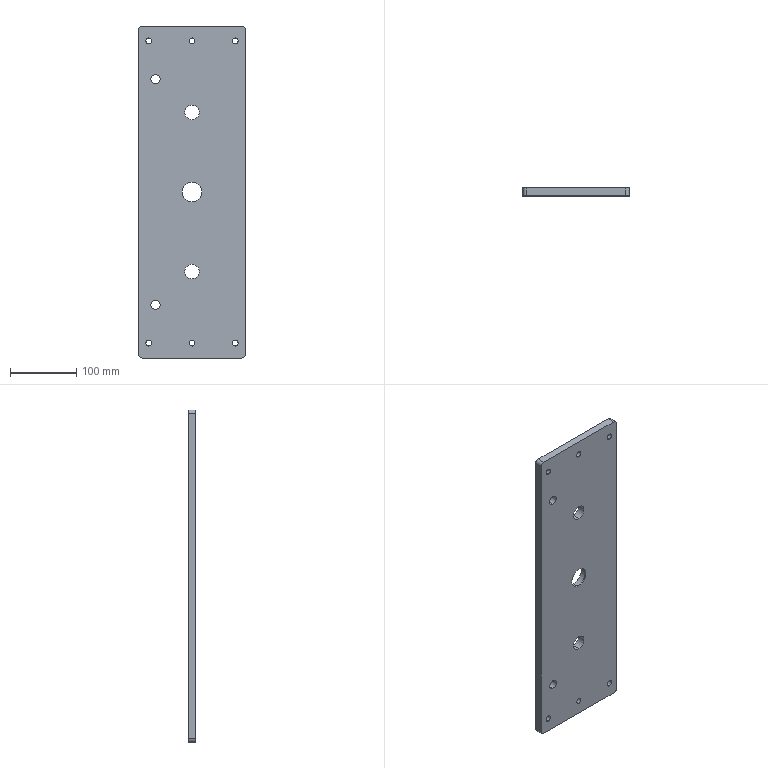Part | SolidWorks | features ICE 3, Extrusion 1, Fillet 1, HoleWzd 1 | 1 solid | 35 faces | box 160 x 12 x 500 mm | volume 931309 mm3 | cylinder 28 | plane 7 | commonest cylinder face diameters 9 x12 10 x4 14 x4 22 x4 30 x2 35 x2
STEP:
#1=CARTESIAN_POINT('',(-55.,12.,177.));
#2=VERTEX_POINT('',#1);
#3=CARTESIAN_POINT('',(-55.,12.,163.));
#4=VERTEX_POINT('',#3);
#5=CARTESIAN_POINT('',(-55.,12.,170.));
#6=DIRECTION('',(0.,-1.,0.));
#7=DIRECTION('',(0.,0.,-1.));
#8=AXIS2_PLACEMENT_3D('',#5,#6,#7);
#9=CIRCLE('',#8,7.);
#10=EDGE_CURVE('',#2,#4,#9,.T.);
#11=ORIENTED_EDGE('',*,*,#10,.F.);
#12=CARTESIAN_POINT('',(-55.,0.,177.));
#13=VERTEX_POINT('',#12);
#14=CARTESIAN_POINT('',(-55.,12.,177.));
#15=DIRECTION('',(0.,-1.,0.));
#16=VECTOR('',#15,1000.);
#17=LINE('',#14,#16);
#18=EDGE_CURVE('',#2,#13,#17,.T.);
#19=ORIENTED_EDGE('',*,*,#18,.T.);
#20=CARTESIAN_POINT('',(-55.,0.,163.));
#21=VERTEX_POINT('',#20);
#22=CARTESIAN_POINT('',(-55.,0.,170.));
#23=DIRECTION('',(0.,-1.,0.));
#24=DIRECTION('',(0.,0.,-1.));
#25=AXIS2_PLACEMENT_3D('',#22,#23,#24);
#26=CIRCLE('',#25,7.);
#27=EDGE_CURVE('',#13,#21,#26,.T.);
#28=ORIENTED_EDGE('',*,*,#27,.T.);
#29=CARTESIAN_POINT('',(-55.,12.,163.));
#30=DIRECTION('',(0.,-1.,0.));
#31=VECTOR('',#30,1000.);
#32=LINE('',#29,#31);
#33=EDGE_CURVE('',#4,#21,#32,.T.);
#34=ORIENTED_EDGE('',*,*,#33,.F.);
#35=EDGE_LOOP('',(#11,#19,#28,#34));
#36=FACE_OUTER_BOUND('',#35,.T.);
#37=CARTESIAN_POINT('',(-55.,12.,170.));
#38=DIRECTION('',(0.,-1.,0.));
#39=DIRECTION('',(0.,0.,-1.));
#40=AXIS2_PLACEMENT_3D('',#37,#38,#39);
#41=CYLINDRICAL_SURFACE('',#40,7.);
#42=ADVANCED_FACE('',(#36),#41,.F.);
#43=CARTESIAN_POINT('',(-55.,12.,-163.));
#44=VERTEX_POINT('',#43);
#45=CARTESIAN_POINT('',(-55.,12.,-177.));
#46=VERTEX_POINT('',#45);
#47=CARTESIAN_POINT('',(-55.,12.,-170.));
#48=DIRECTION('',(0.,-1.,0.));
#49=DIRECTION('',(0.,0.,1.));
#50=AXIS2_PLACEMENT_3D('',#47,#48,#49);
#51=CIRCLE('',#50,7.);
#52=EDGE_CURVE('',#44,#46,#51,.T.);
#53=ORIENTED_EDGE('',*,*,#52,.F.);
#54=CARTESIAN_POINT('',(-55.,0.,-163.));
#55=VERTEX_POINT('',#54);
#56=CARTESIAN_POINT('',(-55.,12.,-163.));
#57=DIRECTION('',(0.,-1.,0.));
#58=VECTOR('',#57,1000.);
#59=LINE('',#56,#58);
#60=EDGE_CURVE('',#44,#55,#59,.T.);
#61=ORIENTED_EDGE('',*,*,#60,.T.);
#62=CARTESIAN_POINT('',(-55.,0.,-177.));
#63=VERTEX_POINT('',#62);
#64=CARTESIAN_POINT('',(-55.,0.,-170.));
#65=DIRECTION('',(0.,-1.,0.));
#66=DIRECTION('',(0.,0.,1.));
#67=AXIS2_PLACEMENT_3D('',#64,#65,#66);
#68=CIRCLE('',#67,7.);
#69=EDGE_CURVE('',#55,#63,#68,.T.);
#70=ORIENTED_EDGE('',*,*,#69,.T.);
#71=CARTESIAN_POINT('',(-55.,12.,-177.));
#72=DIRECTION('',(0.,-1.,0.));
#73=VECTOR('',#72,1000.);
#74=LINE('',#71,#73);
#75=EDGE_CURVE('',#46,#63,#74,.T.);
#76=ORIENTED_EDGE('',*,*,#75,.F.);
#77=EDGE_LOOP('',(#53,#61,#70,#76));
#78=FACE_OUTER_BOUND('',#77,.T.);
#79=CARTESIAN_POINT('',(-55.,12.,-170.));
#80=DIRECTION('',(0.,-1.,0.));
#81=DIRECTION('',(0.,0.,-1.));
#82=AXIS2_PLACEMENT_3D('',#79,#80,#81);
#83=CYLINDRICAL_SURFACE('',#82,7.);
#84=ADVANCED_FACE('',(#78),#83,.F.);
#85=CARTESIAN_POINT('',(-65.,0.,-223.));
#86=VERTEX_POINT('',#85);
#87=CARTESIAN_POINT('',(-65.,0.,-232.));
#88=VERTEX_POINT('',#87);
#89=CARTESIAN_POINT('',(-65.,0.,-227.5));
#90=DIRECTION('',(0.,-1.,0.));
#91=DIRECTION('',(0.,0.,-1.));
#92=AXIS2_PLACEMENT_3D('',#89,#90,#91);
#93=CIRCLE('',#92,4.5);
#94=EDGE_CURVE('',#86,#88,#93,.T.);
#95=ORIENTED_EDGE('',*,*,#94,.T.);
#96=CARTESIAN_POINT('',(-65.,12.,-232.));
#97=VERTEX_POINT('',#96);
#98=CARTESIAN_POINT('',(-65.,12.,-232.));
#99=DIRECTION('',(0.,1.,0.));
#100=VECTOR('',#99,1000.);
#101=LINE('',#98,#100);
#102=EDGE_CURVE('',#88,#97,#101,.T.);
#103=ORIENTED_EDGE('',*,*,#102,.T.);
#104=CARTESIAN_POINT('',(-65.,12.,-223.));
#105=VERTEX_POINT('',#104);
#106=CARTESIAN_POINT('',(-65.,12.,-227.5));
#107=DIRECTION('',(0.,1.,0.));
#108=DIRECTION('',(0.,0.,1.));
#109=AXIS2_PLACEMENT_3D('',#106,#107,#108);
#110=CIRCLE('',#109,4.5);
#111=EDGE_CURVE('',#97,#105,#110,.T.);
#112=ORIENTED_EDGE('',*,*,#111,.T.);
#113=CARTESIAN_POINT('',(-65.,12.,-223.));
#114=DIRECTION('',(0.,1.,0.));
#115=VECTOR('',#114,1000.);
#116=LINE('',#113,#115);
#117=EDGE_CURVE('',#86,#105,#116,.T.);
#118=ORIENTED_EDGE('',*,*,#117,.F.);
#119=EDGE_LOOP('',(#95,#103,#112,#118));
#120=FACE_OUTER_BOUND('',#119,.T.);
#121=CARTESIAN_POINT('',(-65.,12.,-227.5));
#122=DIRECTION('',(0.,1.,0.));
#123=DIRECTION('',(0.,0.,1.));
#124=AXIS2_PLACEMENT_3D('',#121,#122,#123);
#125=CYLINDRICAL_SURFACE('',#124,4.5);
#126=ADVANCED_FACE('',(#120),#125,.F.);
#127=CARTESIAN_POINT('',(0.,0.,-223.));
#128=VERTEX_POINT('',#127);
#129=CARTESIAN_POINT('',(0.,0.,-232.));
#130=VERTEX_POINT('',#129);
#131=CARTESIAN_POINT('',(0.,0.,-227.5));
#132=DIRECTION('',(0.,-1.,0.));
#133=DIRECTION('',(0.,0.,-1.));
#134=AXIS2_PLACEMENT_3D('',#131,#132,#133);
#135=CIRCLE('',#134,4.5);
#136=EDGE_CURVE('',#128,#130,#135,.T.);
#137=ORIENTED_EDGE('',*,*,#136,.T.);
#138=CARTESIAN_POINT('',(0.,12.,-232.));
#139=VERTEX_POINT('',#138);
#140=CARTESIAN_POINT('',(0.,12.,-232.));
#141=DIRECTION('',(0.,1.,0.));
#142=VECTOR('',#141,1000.);
#143=LINE('',#140,#142);
#144=EDGE_CURVE('',#130,#139,#143,.T.);
#145=ORIENTED_EDGE('',*,*,#144,.T.);
#146=CARTESIAN_POINT('',(0.,12.,-223.));
#147=VERTEX_POINT('',#146);
#148=CARTESIAN_POINT('',(0.,12.,-227.5));
#149=DIRECTION('',(0.,1.,0.));
#150=DIRECTION('',(0.,0.,1.));
#151=AXIS2_PLACEMENT_3D('',#148,#149,#150);
#152=CIRCLE('',#151,4.5);
#153=EDGE_CURVE('',#139,#147,#152,.T.);
#154=ORIENTED_EDGE('',*,*,#153,.T.);
#155=CARTESIAN_POINT('',(0.,12.,-223.));
#156=DIRECTION('',(0.,1.,0.));
#157=VECTOR('',#156,1000.);
#158=LINE('',#155,#157);
#159=EDGE_CURVE('',#128,#147,#158,.T.);
#160=ORIENTED_EDGE('',*,*,#159,.F.);
#161=EDGE_LOOP('',(#137,#145,#154,#160));
#162=FACE_OUTER_BOUND('',#161,.T.);
#163=CARTESIAN_POINT('',(0.,12.,-227.5));
#164=DIRECTION('',(0.,1.,0.));
#165=DIRECTION('',(0.,0.,1.));
#166=AXIS2_PLACEMENT_3D('',#163,#164,#165);
#167=CYLINDRICAL_SURFACE('',#166,4.5);
#168=ADVANCED_FACE('',(#162),#167,.F.);
#169=CARTESIAN_POINT('',(65.,0.,-223.));
#170=VERTEX_POINT('',#169);
#171=CARTESIAN_POINT('',(65.,0.,-232.));
#172=VERTEX_POINT('',#171);
#173=CARTESIAN_POINT('',(65.,0.,-227.5));
#174=DIRECTION('',(0.,-1.,0.));
#175=DIRECTION('',(0.,0.,-1.));
#176=AXIS2_PLACEMENT_3D('',#173,#174,#175);
#177=CIRCLE('',#176,4.5);
#178=EDGE_CURVE('',#170,#172,#177,.T.);
#179=ORIENTED_EDGE('',*,*,#178,.T.);
#180=CARTESIAN_POINT('',(65.,12.,-232.));
#181=VERTEX_POINT('',#180);
#182=CARTESIAN_POINT('',(65.,12.,-232.));
#183=DIRECTION('',(0.,1.,0.));
#184=VECTOR('',#183,1000.);
#185=LINE('',#182,#184);
#186=EDGE_CURVE('',#172,#181,#185,.T.);
#187=ORIENTED_EDGE('',*,*,#186,.T.);
#188=CARTESIAN_POINT('',(65.,12.,-223.));
#189=VERTEX_POINT('',#188);
#190=CARTESIAN_POINT('',(65.,12.,-227.5));
#191=DIRECTION('',(0.,1.,0.));
#192=DIRECTION('',(0.,0.,1.));
#193=AXIS2_PLACEMENT_3D('',#190,#191,#192);
#194=CIRCLE('',#193,4.5);
#195=EDGE_CURVE('',#181,#189,#194,.T.);
#196=ORIENTED_EDGE('',*,*,#195,.T.);
#197=CARTESIAN_POINT('',(65.,12.,-223.));
#198=DIRECTION('',(0.,1.,0.));
#199=VECTOR('',#198,1000.);
#200=LINE('',#197,#199);
#201=EDGE_CURVE('',#170,#189,#200,.T.);
#202=ORIENTED_EDGE('',*,*,#201,.F.);
#203=EDGE_LOOP('',(#179,#187,#196,#202));
#204=FACE_OUTER_BOUND('',#203,.T.);
#205=CARTESIAN_POINT('',(65.,12.,-227.5));
#206=DIRECTION('',(0.,1.,0.));
#207=DIRECTION('',(0.,0.,1.));
#208=AXIS2_PLACEMENT_3D('',#205,#206,#207);
#209=CYLINDRICAL_SURFACE('',#208,4.5);
#210=ADVANCED_FACE('',(#204),#209,.F.);
#211=CARTESIAN_POINT('',(-65.,0.,232.));
#212=VERTEX_POINT('',#211);
#213=CARTESIAN_POINT('',(-65.,0.,223.));
#214=VERTEX_POINT('',#213);
#215=CARTESIAN_POINT('',(-65.,0.,227.5));
#216=DIRECTION('',(0.,-1.,0.));
#217=DIRECTION('',(0.,0.,-1.));
#218=AXIS2_PLACEMENT_3D('',#215,#216,#217);
#219=CIRCLE('',#218,4.5);
#220=EDGE_CURVE('',#212,#214,#219,.T.);
#221=ORIENTED_EDGE('',*,*,#220,.T.);
#222=CARTESIAN_POINT('',(-65.,12.,223.));
#223=VERTEX_POINT('',#222);
#224=CARTESIAN_POINT('',(-65.,12.,223.));
#225=DIRECTION('',(0.,1.,0.));
#226=VECTOR('',#225,1000.);
#227=LINE('',#224,#226);
#228=EDGE_CURVE('',#214,#223,#227,.T.);
#229=ORIENTED_EDGE('',*,*,#228,.T.);
#230=CARTESIAN_POINT('',(-65.,12.,232.));
#231=VERTEX_POINT('',#230);
#232=CARTESIAN_POINT('',(-65.,12.,227.5));
#233=DIRECTION('',(0.,1.,0.));
#234=DIRECTION('',(0.,0.,1.));
#235=AXIS2_PLACEMENT_3D('',#232,#233,#234);
#236=CIRCLE('',#235,4.5);
#237=EDGE_CURVE('',#223,#231,#236,.T.);
#238=ORIENTED_EDGE('',*,*,#237,.T.);
#239=CARTESIAN_POINT('',(-65.,12.,232.));
#240=DIRECTION('',(0.,1.,0.));
#241=VECTOR('',#240,1000.);
#242=LINE('',#239,#241);
#243=EDGE_CURVE('',#212,#231,#242,.T.);
#244=ORIENTED_EDGE('',*,*,#243,.F.);
#245=EDGE_LOOP('',(#221,#229,#238,#244));
#246=FACE_OUTER_BOUND('',#245,.T.);
#247=CARTESIAN_POINT('',(-65.,12.,227.5));
#248=DIRECTION('',(0.,1.,0.));
#249=DIRECTION('',(0.,0.,1.));
#250=AXIS2_PLACEMENT_3D('',#247,#248,#249);
#251=CYLINDRICAL_SURFACE('',#250,4.5);
#252=ADVANCED_FACE('',(#246),#251,.F.);
#253=CARTESIAN_POINT('',(0.,0.,232.));
#254=VERTEX_POINT('',#253);
#255=CARTESIAN_POINT('',(0.,0.,223.));
#256=VERTEX_POINT('',#255);
#257=CARTESIAN_POINT('',(0.,0.,227.5));
#258=DIRECTION('',(0.,-1.,0.));
#259=DIRECTION('',(0.,0.,-1.));
#260=AXIS2_PLACEMENT_3D('',#257,#258,#259);
#261=CIRCLE('',#260,4.5);
#262=EDGE_CURVE('',#254,#256,#261,.T.);
#263=ORIENTED_EDGE('',*,*,#262,.T.);
#264=CARTESIAN_POINT('',(0.,12.,223.));
#265=VERTEX_POINT('',#264);
#266=CARTESIAN_POINT('',(0.,12.,223.));
#267=DIRECTION('',(0.,1.,0.));
#268=VECTOR('',#267,1000.);
#269=LINE('',#266,#268);
#270=EDGE_CURVE('',#256,#265,#269,.T.);
#271=ORIENTED_EDGE('',*,*,#270,.T.);
#272=CARTESIAN_POINT('',(0.,12.,232.));
#273=VERTEX_POINT('',#272);
#274=CARTESIAN_POINT('',(0.,12.,227.5));
#275=DIRECTION('',(0.,1.,0.));
#276=DIRECTION('',(0.,0.,1.));
#277=AXIS2_PLACEMENT_3D('',#274,#275,#276);
#278=CIRCLE('',#277,4.5);
#279=EDGE_CURVE('',#265,#273,#278,.T.);
#280=ORIENTED_EDGE('',*,*,#279,.T.);
#281=CARTESIAN_POINT('',(0.,12.,232.));
#282=DIRECTION('',(0.,1.,0.));
#283=VECTOR('',#282,1000.);
#284=LINE('',#281,#283);
#285=EDGE_CURVE('',#254,#273,#284,.T.);
#286=ORIENTED_EDGE('',*,*,#285,.F.);
#287=EDGE_LOOP('',(#263,#271,#280,#286));
#288=FACE_OUTER_BOUND('',#287,.T.);
#289=CARTESIAN_POINT('',(0.,12.,227.5));
#290=DIRECTION('',(0.,1.,0.));
#291=DIRECTION('',(0.,0.,1.));
#292=AXIS2_PLACEMENT_3D('',#289,#290,#291);
#293=CYLINDRICAL_SURFACE('',#292,4.5);
#294=ADVANCED_FACE('',(#288),#293,.F.);
#295=CARTESIAN_POINT('',(65.,0.,232.));
#296=VERTEX_POINT('',#295);
#297=CARTESIAN_POINT('',(65.,0.,223.));
#298=VERTEX_POINT('',#297);
#299=CARTESIAN_POINT('',(65.,0.,227.5));
#300=DIRECTION('',(0.,-1.,0.));
#301=DIRECTION('',(0.,0.,-1.));
#302=AXIS2_PLACEMENT_3D('',#299,#300,#301);
#303=CIRCLE('',#302,4.5);
#304=EDGE_CURVE('',#296,#298,#303,.T.);
#305=ORIENTED_EDGE('',*,*,#304,.T.);
#306=CARTESIAN_POINT('',(65.,12.,223.));
#307=VERTEX_POINT('',#306);
#308=CARTESIAN_POINT('',(65.,12.,223.));
#309=DIRECTION('',(0.,1.,0.));
#310=VECTOR('',#309,1000.);
#311=LINE('',#308,#310);
#312=EDGE_CURVE('',#298,#307,#311,.T.);
#313=ORIENTED_EDGE('',*,*,#312,.T.);
#314=CARTESIAN_POINT('',(65.,12.,232.));
#315=VERTEX_POINT('',#314);
#316=CARTESIAN_POINT('',(65.,12.,227.5));
#317=DIRECTION('',(0.,1.,0.));
#318=DIRECTION('',(0.,0.,1.));
#319=AXIS2_PLACEMENT_3D('',#316,#317,#318);
#320=CIRCLE('',#319,4.5);
#321=EDGE_CURVE('',#307,#315,#320,.T.);
#322=ORIENTED_EDGE('',*,*,#321,.T.);
#323=CARTESIAN_POINT('',(65.,12.,232.));
#324=DIRECTION('',(0.,1.,0.));
#325=VECTOR('',#324,1000.);
#326=LINE('',#323,#325);
#327=EDGE_CURVE('',#296,#315,#326,.T.);
#328=ORIENTED_EDGE('',*,*,#327,.F.);
#329=EDGE_LOOP('',(#305,#313,#322,#328));
#330=FACE_OUTER_BOUND('',#329,.T.);
#331=CARTESIAN_POINT('',(65.,12.,227.5));
#332=DIRECTION('',(0.,1.,0.));
#333=DIRECTION('',(0.,0.,1.));
#334=AXIS2_PLACEMENT_3D('',#331,#332,#333);
#335=CYLINDRICAL_SURFACE('',#334,4.5);
#336=ADVANCED_FACE('',(#330),#335,.F.);
#337=CARTESIAN_POINT('',(0.,2.,-17.5));
#338=VERTEX_POINT('',#337);
#339=CARTESIAN_POINT('',(0.,2.,17.5));
#340=VERTEX_POINT('',#339);
#341=CARTESIAN_POINT('',(0.,2.,0.));
#342=DIRECTION('',(0.,1.,0.));
#343=DIRECTION('',(0.,0.,1.));
#344=AXIS2_PLACEMENT_3D('',#341,#342,#343);
#345=CIRCLE('',#344,17.5);
#346=EDGE_CURVE('',#338,#340,#345,.T.);
#347=ORIENTED_EDGE('',*,*,#346,.F.);
#348=CARTESIAN_POINT('',(0.,12.,-17.5));
#349=VERTEX_POINT('',#348);
#350=CARTESIAN_POINT('',(0.,2.,-17.5));
#351=DIRECTION('',(0.,1.,0.));
#352=VECTOR('',#351,1000.);
#353=LINE('',#350,#352);
#354=EDGE_CURVE('',#338,#349,#353,.T.);
#355=ORIENTED_EDGE('',*,*,#354,.T.);
#356=CARTESIAN_POINT('',(0.,12.,17.5));
#357=VERTEX_POINT('',#356);
#358=CARTESIAN_POINT('',(0.,12.,0.));
#359=DIRECTION('',(0.,1.,0.));
#360=DIRECTION('',(0.,0.,1.));
#361=AXIS2_PLACEMENT_3D('',#358,#359,#360);
#362=CIRCLE('',#361,17.5);
#363=EDGE_CURVE('',#349,#357,#362,.T.);
#364=ORIENTED_EDGE('',*,*,#363,.T.);
#365=CARTESIAN_POINT('',(0.,2.,17.5));
#366=DIRECTION('',(0.,1.,0.));
#367=VECTOR('',#366,1000.);
#368=LINE('',#365,#367);
#369=EDGE_CURVE('',#340,#357,#368,.T.);
#370=ORIENTED_EDGE('',*,*,#369,.F.);
#371=EDGE_LOOP('',(#347,#355,#364,#370));
#372=FACE_OUTER_BOUND('',#371,.T.);
#373=CARTESIAN_POINT('',(0.,2.,0.));
#374=DIRECTION('',(0.,1.,0.));
#375=DIRECTION('',(0.,0.,1.));
#376=AXIS2_PLACEMENT_3D('',#373,#374,#375);
#377=CYLINDRICAL_SURFACE('',#376,17.5);
#378=ADVANCED_FACE('',(#372),#377,.F.);
#379=CARTESIAN_POINT('',(0.,0.,109.));
#380=VERTEX_POINT('',#379);
#381=CARTESIAN_POINT('',(0.,0.,131.));
#382=VERTEX_POINT('',#381);
#383=CARTESIAN_POINT('',(0.,0.,120.));
#384=DIRECTION('',(0.,1.,0.));
#385=DIRECTION('',(0.,0.,1.));
#386=AXIS2_PLACEMENT_3D('',#383,#384,#385);
#387=CIRCLE('',#386,11.);
#388=EDGE_CURVE('',#380,#382,#387,.T.);
#389=ORIENTED_EDGE('',*,*,#388,.F.);
#390=CARTESIAN_POINT('',(0.,12.,109.));
#391=VERTEX_POINT('',#390);
#392=CARTESIAN_POINT('',(0.,0.,109.));
#393=DIRECTION('',(0.,1.,0.));
#394=VECTOR('',#393,1000.);
#395=LINE('',#392,#394);
#396=EDGE_CURVE('',#380,#391,#395,.T.);
#397=ORIENTED_EDGE('',*,*,#396,.T.);
#398=CARTESIAN_POINT('',(0.,12.,131.));
#399=VERTEX_POINT('',#398);
#400=CARTESIAN_POINT('',(0.,12.,120.));
#401=DIRECTION('',(0.,1.,0.));
#402=DIRECTION('',(0.,0.,1.));
#403=AXIS2_PLACEMENT_3D('',#400,#401,#402);
#404=CIRCLE('',#403,11.);
#405=EDGE_CURVE('',#391,#399,#404,.T.);
#406=ORIENTED_EDGE('',*,*,#405,.T.);
#407=CARTESIAN_POINT('',(0.,0.,131.));
#408=DIRECTION('',(0.,1.,0.));
#409=VECTOR('',#408,1000.);
#410=LINE('',#407,#409);
#411=EDGE_CURVE('',#382,#399,#410,.T.);
#412=ORIENTED_EDGE('',*,*,#411,.F.);
#413=EDGE_LOOP('',(#389,#397,#406,#412));
#414=FACE_OUTER_BOUND('',#413,.T.);
#415=CARTESIAN_POINT('',(0.,0.,120.));
#416=DIRECTION('',(0.,1.,0.));
#417=DIRECTION('',(0.,0.,1.));
#418=AXIS2_PLACEMENT_3D('',#415,#416,#417);
#419=CYLINDRICAL_SURFACE('',#418,11.);
#420=ADVANCED_FACE('',(#414),#419,.F.);
#421=CARTESIAN_POINT('',(0.,0.,-131.));
#422=VERTEX_POINT('',#421);
#423=CARTESIAN_POINT('',(0.,0.,-109.));
#424=VERTEX_POINT('',#423);
#425=CARTESIAN_POINT('',(0.,0.,-120.));
#426=DIRECTION('',(0.,1.,0.));
#427=DIRECTION('',(0.,0.,-1.));
#428=AXIS2_PLACEMENT_3D('',#425,#426,#427);
#429=CIRCLE('',#428,11.);
#430=EDGE_CURVE('',#422,#424,#429,.T.);
#431=ORIENTED_EDGE('',*,*,#430,.F.);
#432=CARTESIAN_POINT('',(0.,12.,-131.));
#433=VERTEX_POINT('',#432);
#434=CARTESIAN_POINT('',(0.,0.,-131.));
#435=DIRECTION('',(0.,1.,0.));
#436=VECTOR('',#435,1000.);
#437=LINE('',#434,#436);
#438=EDGE_CURVE('',#422,#433,#437,.T.);
#439=ORIENTED_EDGE('',*,*,#438,.T.);
#440=CARTESIAN_POINT('',(0.,12.,-109.));
#441=VERTEX_POINT('',#440);
#442=CARTESIAN_POINT('',(0.,12.,-120.));
#443=DIRECTION('',(0.,1.,0.));
#444=DIRECTION('',(0.,0.,-1.));
#445=AXIS2_PLACEMENT_3D('',#442,#443,#444);
#446=CIRCLE('',#445,11.);
#447=EDGE_CURVE('',#433,#441,#446,.T.);
#448=ORIENTED_EDGE('',*,*,#447,.T.);
#449=CARTESIAN_POINT('',(0.,0.,-109.));
#450=DIRECTION('',(0.,1.,0.));
#451=VECTOR('',#450,1000.);
#452=LINE('',#449,#451);
#453=EDGE_CURVE('',#424,#441,#452,.T.);
#454=ORIENTED_EDGE('',*,*,#453,.F.);
#455=EDGE_LOOP('',(#431,#439,#448,#454));
#456=FACE_OUTER_BOUND('',#455,.T.);
#457=CARTESIAN_POINT('',(0.,0.,-120.));
#458=DIRECTION('',(0.,1.,0.));
#459=DIRECTION('',(0.,0.,1.));
#460=AXIS2_PLACEMENT_3D('',#457,#458,#459);
#461=CYLINDRICAL_SURFACE('',#460,11.);
#462=ADVANCED_FACE('',(#456),#461,.F.);
#463=CARTESIAN_POINT('',(0.,0.,-15.));
#464=VERTEX_POINT('',#463);
#465=CARTESIAN_POINT('',(0.,0.,15.));
#466=VERTEX_POINT('',#465);
#467=CARTESIAN_POINT('',(0.,0.,0.));
#468=DIRECTION('',(0.,1.,0.));
#469=DIRECTION('',(0.,0.,1.));
#470=AXIS2_PLACEMENT_3D('',#467,#468,#469);
#471=CIRCLE('',#470,15.);
#472=EDGE_CURVE('',#464,#466,#471,.T.);
#473=ORIENTED_EDGE('',*,*,#472,.F.);
#474=CARTESIAN_POINT('',(0.,2.,-15.));
#475=VERTEX_POINT('',#474);
#476=CARTESIAN_POINT('',(0.,0.,-15.));
#477=DIRECTION('',(0.,1.,0.));
#478=VECTOR('',#477,1000.);
#479=LINE('',#476,#478);
#480=EDGE_CURVE('',#464,#475,#479,.T.);
#481=ORIENTED_EDGE('',*,*,#480,.T.);
#482=CARTESIAN_POINT('',(0.,2.,15.));
#483=VERTEX_POINT('',#482);
#484=CARTESIAN_POINT('',(0.,2.,0.));
#485=DIRECTION('',(0.,-1.,0.));
#486=DIRECTION('',(0.,0.,1.));
#487=AXIS2_PLACEMENT_3D('',#484,#485,#486);
#488=CIRCLE('',#487,15.);
#489=EDGE_CURVE('',#483,#475,#488,.T.);
#490=ORIENTED_EDGE('',*,*,#489,.F.);
#491=CARTESIAN_POINT('',(0.,0.,15.));
#492=DIRECTION('',(0.,1.,0.));
#493=VECTOR('',#492,1000.);
#494=LINE('',#491,#493);
#495=EDGE_CURVE('',#466,#483,#494,.T.);
#496=ORIENTED_EDGE('',*,*,#495,.F.);
#497=EDGE_LOOP('',(#473,#481,#490,#496));
#498=FACE_OUTER_BOUND('',#497,.T.);
#499=CARTESIAN_POINT('',(0.,0.,0.));
#500=DIRECTION('',(0.,1.,0.));
#501=DIRECTION('',(0.,0.,1.));
#502=AXIS2_PLACEMENT_3D('',#499,#500,#501);
#503=CYLINDRICAL_SURFACE('',#502,15.);
#504=ADVANCED_FACE('',(#498),#503,.F.);
#505=ORIENTED_EDGE('',*,*,#480,.F.);
#506=CARTESIAN_POINT('',(0.,0.,0.));
#507=DIRECTION('',(0.,1.,0.));
#508=DIRECTION('',(0.,0.,1.));
#509=AXIS2_PLACEMENT_3D('',#506,#507,#508);
#510=CIRCLE('',#509,15.);
#511=EDGE_CURVE('',#466,#464,#510,.T.);
#512=ORIENTED_EDGE('',*,*,#511,.F.);
#513=ORIENTED_EDGE('',*,*,#495,.T.);
#514=CARTESIAN_POINT('',(0.,2.,0.));
#515=DIRECTION('',(0.,-1.,0.));
#516=DIRECTION('',(0.,0.,1.));
#517=AXIS2_PLACEMENT_3D('',#514,#515,#516);
#518=CIRCLE('',#517,15.);
#519=EDGE_CURVE('',#475,#483,#518,.T.);
#520=ORIENTED_EDGE('',*,*,#519,.F.);
#521=EDGE_LOOP('',(#505,#512,#513,#520));
#522=FACE_OUTER_BOUND('',#521,.T.);
#523=CARTESIAN_POINT('',(0.,0.,0.));
#524=DIRECTION('',(0.,1.,0.));
#525=DIRECTION('',(0.,0.,1.));
#526=AXIS2_PLACEMENT_3D('',#523,#524,#525);
#527=CYLINDRICAL_SURFACE('',#526,15.);
#528=ADVANCED_FACE('',(#522),#527,.F.);
#529=CARTESIAN_POINT('',(80.,0.,245.));
#530=VERTEX_POINT('',#529);
#531=CARTESIAN_POINT('',(80.,0.,-245.));
#532=VERTEX_POINT('',#531);
#533=CARTESIAN_POINT('',(80.,0.,250.));
#534=DIRECTION('',(0.,0.,-1.));
#535=VECTOR('',#534,1000.);
#536=LINE('',#533,#535);
#537=EDGE_CURVE('',#530,#532,#536,.T.);
#538=ORIENTED_EDGE('',*,*,#537,.T.);
#539=CARTESIAN_POINT('',(80.,12.,-245.));
#540=VERTEX_POINT('',#539);
#541=CARTESIAN_POINT('',(80.,12.,-245.));
#542=DIRECTION('',(0.,1.,0.));
#543=VECTOR('',#542,1000.);
#544=LINE('',#541,#543);
#545=EDGE_CURVE('',#532,#540,#544,.T.);
#546=ORIENTED_EDGE('',*,*,#545,.T.);
#547=CARTESIAN_POINT('',(80.,12.,245.));
#548=VERTEX_POINT('',#547);
#549=CARTESIAN_POINT('',(80.,12.,250.));
#550=DIRECTION('',(0.,0.,-1.));
#551=VECTOR('',#550,1000.);
#552=LINE('',#549,#551);
#553=EDGE_CURVE('',#548,#540,#552,.T.);
#554=ORIENTED_EDGE('',*,*,#553,.F.);
#555=CARTESIAN_POINT('',(80.,12.,245.));
#556=DIRECTION('',(0.,-1.,0.));
#557=VECTOR('',#556,1000.);
#558=LINE('',#555,#557);
#559=EDGE_CURVE('',#548,#530,#558,.T.);
#560=ORIENTED_EDGE('',*,*,#559,.T.);
#561=EDGE_LOOP('',(#538,#546,#554,#560));
#562=FACE_OUTER_BOUND('',#561,.T.);
#563=CARTESIAN_POINT('',(80.,12.,250.));
#564=DIRECTION('',(-1.,0.,0.));
#565=DIRECTION('',(0.,0.,1.));
#566=AXIS2_PLACEMENT_3D('',#563,#564,#565);
#567=PLANE('',#566);
#568=ADVANCED_FACE('',(#562),#567,.F.);
#569=CARTESIAN_POINT('',(75.,0.,-250.));
#570=VERTEX_POINT('',#569);
#571=CARTESIAN_POINT('',(-75.,0.,-250.));
#572=VERTEX_POINT('',#571);
#573=CARTESIAN_POINT('',(-80.,0.,-250.));
#574=DIRECTION('',(-1.,0.,0.));
#575=VECTOR('',#574,1000.);
#576=LINE('',#573,#575);
#577=EDGE_CURVE('',#570,#572,#576,.T.);
#578=ORIENTED_EDGE('',*,*,#577,.T.);
#579=CARTESIAN_POINT('',(-75.,12.,-250.));
#580=VERTEX_POINT('',#579);
#581=CARTESIAN_POINT('',(-75.,12.,-250.));
#582=DIRECTION('',(0.,1.,0.));
#583=VECTOR('',#582,1000.);
#584=LINE('',#581,#583);
#585=EDGE_CURVE('',#572,#580,#584,.T.);
#586=ORIENTED_EDGE('',*,*,#585,.T.);
#587=CARTESIAN_POINT('',(75.,12.,-250.));
#588=VERTEX_POINT('',#587);
#589=CARTESIAN_POINT('',(-80.,12.,-250.));
#590=DIRECTION('',(-1.,0.,0.));
#591=VECTOR('',#590,1000.);
#592=LINE('',#589,#591);
#593=EDGE_CURVE('',#588,#580,#592,.T.);
#594=ORIENTED_EDGE('',*,*,#593,.F.);
#595=CARTESIAN_POINT('',(75.,12.,-250.));
#596=DIRECTION('',(0.,-1.,0.));
#597=VECTOR('',#596,1000.);
#598=LINE('',#595,#597);
#599=EDGE_CURVE('',#588,#570,#598,.T.);
#600=ORIENTED_EDGE('',*,*,#599,.T.);
#601=EDGE_LOOP('',(#578,#586,#594,#600));
#602=FACE_OUTER_BOUND('',#601,.T.);
#603=CARTESIAN_POINT('',(-80.,12.,-250.));
#604=DIRECTION('',(0.,0.,1.));
#605=DIRECTION('',(1.,0.,0.));
#606=AXIS2_PLACEMENT_3D('',#603,#604,#605);
#607=PLANE('',#606);
#608=ADVANCED_FACE('',(#602),#607,.F.);
#609=CARTESIAN_POINT('',(-80.,0.,-245.));
#610=VERTEX_POINT('',#609);
#611=CARTESIAN_POINT('',(-80.,0.,245.));
#612=VERTEX_POINT('',#611);
#613=CARTESIAN_POINT('',(-80.,0.,250.));
#614=DIRECTION('',(0.,0.,1.));
#615=VECTOR('',#614,1000.);
#616=LINE('',#613,#615);
#617=EDGE_CURVE('',#610,#612,#616,.T.);
#618=ORIENTED_EDGE('',*,*,#617,.T.);
#619=CARTESIAN_POINT('',(-80.,12.,245.));
#620=VERTEX_POINT('',#619);
#621=CARTESIAN_POINT('',(-80.,12.,245.));
#622=DIRECTION('',(0.,1.,0.));
#623=VECTOR('',#622,1000.);
#624=LINE('',#621,#623);
#625=EDGE_CURVE('',#612,#620,#624,.T.);
#626=ORIENTED_EDGE('',*,*,#625,.T.);
#627=CARTESIAN_POINT('',(-80.,12.,-245.));
#628=VERTEX_POINT('',#627);
#629=CARTESIAN_POINT('',(-80.,12.,250.));
#630=DIRECTION('',(0.,0.,1.));
#631=VECTOR('',#630,1000.);
#632=LINE('',#629,#631);
#633=EDGE_CURVE('',#628,#620,#632,.T.);
#634=ORIENTED_EDGE('',*,*,#633,.F.);
#635=CARTESIAN_POINT('',(-80.,12.,-245.));
#636=DIRECTION('',(0.,-1.,0.));
#637=VECTOR('',#636,1000.);
#638=LINE('',#635,#637);
#639=EDGE_CURVE('',#628,#610,#638,.T.);
#640=ORIENTED_EDGE('',*,*,#639,.T.);
#641=EDGE_LOOP('',(#618,#626,#634,#640));
#642=FACE_OUTER_BOUND('',#641,.T.);
#643=CARTESIAN_POINT('',(-80.,12.,250.));
#644=DIRECTION('',(1.,0.,0.));
#645=DIRECTION('',(0.,0.,-1.));
#646=AXIS2_PLACEMENT_3D('',#643,#644,#645);
#647=PLANE('',#646);
#648=ADVANCED_FACE('',(#642),#647,.F.);
#649=CARTESIAN_POINT('',(-75.,12.,250.));
#650=VERTEX_POINT('',#649);
#651=CARTESIAN_POINT('',(75.,12.,250.));
#652=VERTEX_POINT('',#651);
#653=CARTESIAN_POINT('',(-80.,12.,250.));
#654=DIRECTION('',(1.,0.,0.));
#655=VECTOR('',#654,1000.);
#656=LINE('',#653,#655);
#657=EDGE_CURVE('',#650,#652,#656,.T.);
#658=ORIENTED_EDGE('',*,*,#657,.F.);
#659=CARTESIAN_POINT('',(-75.,0.,250.));
#660=VERTEX_POINT('',#659);
#661=CARTESIAN_POINT('',(-75.,12.,250.));
#662=DIRECTION('',(0.,-1.,0.));
#663=VECTOR('',#662,1000.);
#664=LINE('',#661,#663);
#665=EDGE_CURVE('',#650,#660,#664,.T.);
#666=ORIENTED_EDGE('',*,*,#665,.T.);
#667=CARTESIAN_POINT('',(75.,0.,250.));
#668=VERTEX_POINT('',#667);
#669=CARTESIAN_POINT('',(-80.,0.,250.));
#670=DIRECTION('',(1.,0.,0.));
#671=VECTOR('',#670,1000.);
#672=LINE('',#669,#671);
#673=EDGE_CURVE('',#660,#668,#672,.T.);
#674=ORIENTED_EDGE('',*,*,#673,.T.);
#675=CARTESIAN_POINT('',(75.,12.,250.));
#676=DIRECTION('',(0.,1.,0.));
#677=VECTOR('',#676,1000.);
#678=LINE('',#675,#677);
#679=EDGE_CURVE('',#668,#652,#678,.T.);
#680=ORIENTED_EDGE('',*,*,#679,.T.);
#681=EDGE_LOOP('',(#658,#666,#674,#680));
#682=FACE_OUTER_BOUND('',#681,.T.);
#683=CARTESIAN_POINT('',(-80.,12.,250.));
#684=DIRECTION('',(0.,0.,-1.));
#685=DIRECTION('',(-1.,0.,0.));
#686=AXIS2_PLACEMENT_3D('',#683,#684,#685);
#687=PLANE('',#686);
#688=ADVANCED_FACE('',(#682),#687,.F.);
#689=CARTESIAN_POINT('',(-55.,12.,170.));
#690=DIRECTION('',(0.,-1.,0.));
#691=DIRECTION('',(0.,0.,-1.));
#692=AXIS2_PLACEMENT_3D('',#689,#690,#691);
#693=CIRCLE('',#692,7.);
#694=EDGE_CURVE('',#4,#2,#693,.T.);
#695=ORIENTED_EDGE('',*,*,#694,.T.);
#696=ORIENTED_EDGE('',*,*,#10,.T.);
#697=EDGE_LOOP('',(#695,#696));
#698=FACE_BOUND('',#697,.T.);
#699=CARTESIAN_POINT('',(-55.,12.,-170.));
#700=DIRECTION('',(0.,-1.,0.));
#701=DIRECTION('',(0.,0.,1.));
#702=AXIS2_PLACEMENT_3D('',#699,#700,#701);
#703=CIRCLE('',#702,7.);
#704=EDGE_CURVE('',#46,#44,#703,.T.);
#705=ORIENTED_EDGE('',*,*,#704,.T.);
#706=ORIENTED_EDGE('',*,*,#52,.T.);
#707=EDGE_LOOP('',(#705,#706));
#708=FACE_BOUND('',#707,.T.);
#709=CARTESIAN_POINT('',(-65.,12.,-227.5));
#710=DIRECTION('',(0.,1.,0.));
#711=DIRECTION('',(0.,0.,1.));
#712=AXIS2_PLACEMENT_3D('',#709,#710,#711);
#713=CIRCLE('',#712,4.5);
#714=EDGE_CURVE('',#105,#97,#713,.T.);
#715=ORIENTED_EDGE('',*,*,#714,.F.);
#716=ORIENTED_EDGE('',*,*,#111,.F.);
#717=EDGE_LOOP('',(#715,#716));
#718=FACE_BOUND('',#717,.T.);
#719=CARTESIAN_POINT('',(0.,12.,-227.5));
#720=DIRECTION('',(0.,1.,0.));
#721=DIRECTION('',(0.,0.,1.));
#722=AXIS2_PLACEMENT_3D('',#719,#720,#721);
#723=CIRCLE('',#722,4.5);
#724=EDGE_CURVE('',#147,#139,#723,.T.);
#725=ORIENTED_EDGE('',*,*,#724,.F.);
#726=ORIENTED_EDGE('',*,*,#153,.F.);
#727=EDGE_LOOP('',(#725,#726));
#728=FACE_BOUND('',#727,.T.);
#729=CARTESIAN_POINT('',(65.,12.,-227.5));
#730=DIRECTION('',(0.,1.,0.));
#731=DIRECTION('',(0.,0.,1.));
#732=AXIS2_PLACEMENT_3D('',#729,#730,#731);
#733=CIRCLE('',#732,4.5);
#734=EDGE_CURVE('',#189,#181,#733,.T.);
#735=ORIENTED_EDGE('',*,*,#734,.F.);
#736=ORIENTED_EDGE('',*,*,#195,.F.);
#737=EDGE_LOOP('',(#735,#736));
#738=FACE_BOUND('',#737,.T.);
#739=CARTESIAN_POINT('',(-65.,12.,227.5));
#740=DIRECTION('',(0.,1.,0.));
#741=DIRECTION('',(0.,0.,1.));
#742=AXIS2_PLACEMENT_3D('',#739,#740,#741);
#743=CIRCLE('',#742,4.5);
#744=EDGE_CURVE('',#231,#223,#743,.T.);
#745=ORIENTED_EDGE('',*,*,#744,.F.);
#746=ORIENTED_EDGE('',*,*,#237,.F.);
#747=EDGE_LOOP('',(#745,#746));
#748=FACE_BOUND('',#747,.T.);
#749=CARTESIAN_POINT('',(0.,12.,227.5));
#750=DIRECTION('',(0.,1.,0.));
#751=DIRECTION('',(0.,0.,1.));
#752=AXIS2_PLACEMENT_3D('',#749,#750,#751);
#753=CIRCLE('',#752,4.5);
#754=EDGE_CURVE('',#273,#265,#753,.T.);
#755=ORIENTED_EDGE('',*,*,#754,.F.);
#756=ORIENTED_EDGE('',*,*,#279,.F.);
#757=EDGE_LOOP('',(#755,#756));
#758=FACE_BOUND('',#757,.T.);
#759=CARTESIAN_POINT('',(65.,12.,227.5));
#760=DIRECTION('',(0.,1.,0.));
#761=DIRECTION('',(0.,0.,1.));
#762=AXIS2_PLACEMENT_3D('',#759,#760,#761);
#763=CIRCLE('',#762,4.5);
#764=EDGE_CURVE('',#315,#307,#763,.T.);
#765=ORIENTED_EDGE('',*,*,#764,.F.);
#766=ORIENTED_EDGE('',*,*,#321,.F.);
#767=EDGE_LOOP('',(#765,#766));
#768=FACE_BOUND('',#767,.T.);
#769=CARTESIAN_POINT('',(0.,12.,0.));
#770=DIRECTION('',(0.,1.,0.));
#771=DIRECTION('',(0.,0.,1.));
#772=AXIS2_PLACEMENT_3D('',#769,#770,#771);
#773=CIRCLE('',#772,17.5);
#774=EDGE_CURVE('',#357,#349,#773,.T.);
#775=ORIENTED_EDGE('',*,*,#774,.F.);
#776=ORIENTED_EDGE('',*,*,#363,.F.);
#777=EDGE_LOOP('',(#775,#776));
#778=FACE_BOUND('',#777,.T.);
#779=CARTESIAN_POINT('',(0.,12.,120.));
#780=DIRECTION('',(0.,1.,0.));
#781=DIRECTION('',(0.,0.,1.));
#782=AXIS2_PLACEMENT_3D('',#779,#780,#781);
#783=CIRCLE('',#782,11.);
#784=EDGE_CURVE('',#399,#391,#783,.T.);
#785=ORIENTED_EDGE('',*,*,#784,.F.);
#786=ORIENTED_EDGE('',*,*,#405,.F.);
#787=EDGE_LOOP('',(#785,#786));
#788=FACE_BOUND('',#787,.T.);
#789=CARTESIAN_POINT('',(0.,12.,-120.));
#790=DIRECTION('',(0.,1.,0.));
#791=DIRECTION('',(0.,0.,-1.));
#792=AXIS2_PLACEMENT_3D('',#789,#790,#791);
#793=CIRCLE('',#792,11.);
#794=EDGE_CURVE('',#441,#433,#793,.T.);
#795=ORIENTED_EDGE('',*,*,#794,.F.);
#796=ORIENTED_EDGE('',*,*,#447,.F.);
#797=EDGE_LOOP('',(#795,#796));
#798=FACE_BOUND('',#797,.T.);
#799=ORIENTED_EDGE('',*,*,#633,.T.);
#800=CARTESIAN_POINT('',(-75.,12.,245.));
#801=DIRECTION('',(0.,1.,0.));
#802=DIRECTION('',(0.,0.,-1.));
#803=AXIS2_PLACEMENT_3D('',#800,#801,#802);
#804=CIRCLE('',#803,5.);
#805=EDGE_CURVE('',#620,#650,#804,.T.);
#806=ORIENTED_EDGE('',*,*,#805,.T.);
#807=ORIENTED_EDGE('',*,*,#657,.T.);
#808=CARTESIAN_POINT('',(75.,12.,245.));
#809=DIRECTION('',(0.,1.,0.));
#810=DIRECTION('',(0.,0.,-1.));
#811=AXIS2_PLACEMENT_3D('',#808,#809,#810);
#812=CIRCLE('',#811,5.);
#813=EDGE_CURVE('',#652,#548,#812,.T.);
#814=ORIENTED_EDGE('',*,*,#813,.T.);
#815=ORIENTED_EDGE('',*,*,#553,.T.);
#816=CARTESIAN_POINT('',(75.,12.,-245.));
#817=DIRECTION('',(0.,1.,0.));
#818=DIRECTION('',(0.,0.,-1.));
#819=AXIS2_PLACEMENT_3D('',#816,#817,#818);
#820=CIRCLE('',#819,5.);
#821=EDGE_CURVE('',#540,#588,#820,.T.);
#822=ORIENTED_EDGE('',*,*,#821,.T.);
#823=ORIENTED_EDGE('',*,*,#593,.T.);
#824=CARTESIAN_POINT('',(-75.,12.,-245.));
#825=DIRECTION('',(0.,1.,0.));
#826=DIRECTION('',(0.,0.,-1.));
#827=AXIS2_PLACEMENT_3D('',#824,#825,#826);
#828=CIRCLE('',#827,5.);
#829=EDGE_CURVE('',#580,#628,#828,.T.);
#830=ORIENTED_EDGE('',*,*,#829,.T.);
#831=EDGE_LOOP('',(#799,#806,#807,#814,#815,#822,#823,#830));
#832=FACE_OUTER_BOUND('',#831,.T.);
#833=CARTESIAN_POINT('',(0.,12.,0.));
#834=DIRECTION('',(0.,-1.,0.));
#835=DIRECTION('',(0.,0.,-1.));
#836=AXIS2_PLACEMENT_3D('',#833,#834,#835);
#837=PLANE('',#836);
#838=ADVANCED_FACE('',(#698,#708,#718,#728,#738,#748,#758,#768,#778,#788,#798,#832),#837,.F.);
#839=CARTESIAN_POINT('',(-55.,0.,170.));
#840=DIRECTION('',(0.,-1.,0.));
#841=DIRECTION('',(0.,0.,-1.));
#842=AXIS2_PLACEMENT_3D('',#839,#840,#841);
#843=CIRCLE('',#842,7.);
#844=EDGE_CURVE('',#21,#13,#843,.T.);
#845=ORIENTED_EDGE('',*,*,#844,.F.);
#846=ORIENTED_EDGE('',*,*,#27,.F.);
#847=EDGE_LOOP('',(#845,#846));
#848=FACE_BOUND('',#847,.T.);
#849=CARTESIAN_POINT('',(-55.,0.,-170.));
#850=DIRECTION('',(0.,-1.,0.));
#851=DIRECTION('',(0.,0.,1.));
#852=AXIS2_PLACEMENT_3D('',#849,#850,#851);
#853=CIRCLE('',#852,7.);
#854=EDGE_CURVE('',#63,#55,#853,.T.);
#855=ORIENTED_EDGE('',*,*,#854,.F.);
#856=ORIENTED_EDGE('',*,*,#69,.F.);
#857=EDGE_LOOP('',(#855,#856));
#858=FACE_BOUND('',#857,.T.);
#859=ORIENTED_EDGE('',*,*,#94,.F.);
#860=CARTESIAN_POINT('',(-65.,0.,-227.5));
#861=DIRECTION('',(0.,-1.,0.));
#862=DIRECTION('',(0.,0.,-1.));
#863=AXIS2_PLACEMENT_3D('',#860,#861,#862);
#864=CIRCLE('',#863,4.5);
#865=EDGE_CURVE('',#88,#86,#864,.T.);
#866=ORIENTED_EDGE('',*,*,#865,.F.);
#867=EDGE_LOOP('',(#859,#866));
#868=FACE_BOUND('',#867,.T.);
#869=ORIENTED_EDGE('',*,*,#136,.F.);
#870=CARTESIAN_POINT('',(0.,0.,-227.5));
#871=DIRECTION('',(0.,-1.,0.));
#872=DIRECTION('',(0.,0.,-1.));
#873=AXIS2_PLACEMENT_3D('',#870,#871,#872);
#874=CIRCLE('',#873,4.5);
#875=EDGE_CURVE('',#130,#128,#874,.T.);
#876=ORIENTED_EDGE('',*,*,#875,.F.);
#877=EDGE_LOOP('',(#869,#876));
#878=FACE_BOUND('',#877,.T.);
#879=ORIENTED_EDGE('',*,*,#178,.F.);
#880=CARTESIAN_POINT('',(65.,0.,-227.5));
#881=DIRECTION('',(0.,-1.,0.));
#882=DIRECTION('',(0.,0.,-1.));
#883=AXIS2_PLACEMENT_3D('',#880,#881,#882);
#884=CIRCLE('',#883,4.5);
#885=EDGE_CURVE('',#172,#170,#884,.T.);
#886=ORIENTED_EDGE('',*,*,#885,.F.);
#887=EDGE_LOOP('',(#879,#886));
#888=FACE_BOUND('',#887,.T.);
#889=ORIENTED_EDGE('',*,*,#220,.F.);
#890=CARTESIAN_POINT('',(-65.,0.,227.5));
#891=DIRECTION('',(0.,-1.,0.));
#892=DIRECTION('',(0.,0.,-1.));
#893=AXIS2_PLACEMENT_3D('',#890,#891,#892);
#894=CIRCLE('',#893,4.5);
#895=EDGE_CURVE('',#214,#212,#894,.T.);
#896=ORIENTED_EDGE('',*,*,#895,.F.);
#897=EDGE_LOOP('',(#889,#896));
#898=FACE_BOUND('',#897,.T.);
#899=ORIENTED_EDGE('',*,*,#262,.F.);
#900=CARTESIAN_POINT('',(0.,0.,227.5));
#901=DIRECTION('',(0.,-1.,0.));
#902=DIRECTION('',(0.,0.,-1.));
#903=AXIS2_PLACEMENT_3D('',#900,#901,#902);
#904=CIRCLE('',#903,4.5);
#905=EDGE_CURVE('',#256,#254,#904,.T.);
#906=ORIENTED_EDGE('',*,*,#905,.F.);
#907=EDGE_LOOP('',(#899,#906));
#908=FACE_BOUND('',#907,.T.);
#909=ORIENTED_EDGE('',*,*,#304,.F.);
#910=CARTESIAN_POINT('',(65.,0.,227.5));
#911=DIRECTION('',(0.,-1.,0.));
#912=DIRECTION('',(0.,0.,-1.));
#913=AXIS2_PLACEMENT_3D('',#910,#911,#912);
#914=CIRCLE('',#913,4.5);
#915=EDGE_CURVE('',#298,#296,#914,.T.);
#916=ORIENTED_EDGE('',*,*,#915,.F.);
#917=EDGE_LOOP('',(#909,#916));
#918=FACE_BOUND('',#917,.T.);
#919=CARTESIAN_POINT('',(0.,0.,120.));
#920=DIRECTION('',(0.,1.,0.));
#921=DIRECTION('',(0.,0.,1.));
#922=AXIS2_PLACEMENT_3D('',#919,#920,#921);
#923=CIRCLE('',#922,11.);
#924=EDGE_CURVE('',#382,#380,#923,.T.);
#925=ORIENTED_EDGE('',*,*,#924,.T.);
#926=ORIENTED_EDGE('',*,*,#388,.T.);
#927=EDGE_LOOP('',(#925,#926));
#928=FACE_BOUND('',#927,.T.);
#929=CARTESIAN_POINT('',(0.,0.,-120.));
#930=DIRECTION('',(0.,1.,0.));
#931=DIRECTION('',(0.,0.,-1.));
#932=AXIS2_PLACEMENT_3D('',#929,#930,#931);
#933=CIRCLE('',#932,11.);
#934=EDGE_CURVE('',#424,#422,#933,.T.);
#935=ORIENTED_EDGE('',*,*,#934,.T.);
#936=ORIENTED_EDGE('',*,*,#430,.T.);
#937=EDGE_LOOP('',(#935,#936));
#938=FACE_BOUND('',#937,.T.);
#939=ORIENTED_EDGE('',*,*,#511,.T.);
#940=ORIENTED_EDGE('',*,*,#472,.T.);
#941=EDGE_LOOP('',(#939,#940));
#942=FACE_BOUND('',#941,.T.);
#943=ORIENTED_EDGE('',*,*,#673,.F.);
#944=CARTESIAN_POINT('',(-75.,0.,245.));
#945=DIRECTION('',(0.,-1.,0.));
#946=DIRECTION('',(0.,0.,-1.));
#947=AXIS2_PLACEMENT_3D('',#944,#945,#946);
#948=CIRCLE('',#947,5.);
#949=EDGE_CURVE('',#660,#612,#948,.T.);
#950=ORIENTED_EDGE('',*,*,#949,.T.);
#951=ORIENTED_EDGE('',*,*,#617,.F.);
#952=CARTESIAN_POINT('',(-75.,0.,-245.));
#953=DIRECTION('',(0.,-1.,0.));
#954=DIRECTION('',(0.,0.,-1.));
#955=AXIS2_PLACEMENT_3D('',#952,#953,#954);
#956=CIRCLE('',#955,5.);
#957=EDGE_CURVE('',#610,#572,#956,.T.);
#958=ORIENTED_EDGE('',*,*,#957,.T.);
#959=ORIENTED_EDGE('',*,*,#577,.F.);
#960=CARTESIAN_POINT('',(75.,0.,-245.));
#961=DIRECTION('',(0.,-1.,0.));
#962=DIRECTION('',(0.,0.,-1.));
#963=AXIS2_PLACEMENT_3D('',#960,#961,#962);
#964=CIRCLE('',#963,5.);
#965=EDGE_CURVE('',#570,#532,#964,.T.);
#966=ORIENTED_EDGE('',*,*,#965,.T.);
#967=ORIENTED_EDGE('',*,*,#537,.F.);
#968=CARTESIAN_POINT('',(75.,0.,245.));
#969=DIRECTION('',(0.,-1.,0.));
#970=DIRECTION('',(0.,0.,-1.));
#971=AXIS2_PLACEMENT_3D('',#968,#969,#970);
#972=CIRCLE('',#971,5.);
#973=EDGE_CURVE('',#530,#668,#972,.T.);
#974=ORIENTED_EDGE('',*,*,#973,.T.);
#975=EDGE_LOOP('',(#943,#950,#951,#958,#959,#966,#967,#974));
#976=FACE_OUTER_BOUND('',#975,.T.);
#977=CARTESIAN_POINT('',(0.,0.,0.));
#978=DIRECTION('',(0.,-1.,0.));
#979=DIRECTION('',(0.,0.,-1.));
#980=AXIS2_PLACEMENT_3D('',#977,#978,#979);
#981=PLANE('',#980);
#982=ADVANCED_FACE('',(#848,#858,#868,#878,#888,#898,#908,#918,#928,#938,#942,#976),#981,.T.);
#983=ORIENTED_EDGE('',*,*,#438,.F.);
#984=ORIENTED_EDGE('',*,*,#934,.F.);
#985=ORIENTED_EDGE('',*,*,#453,.T.);
#986=ORIENTED_EDGE('',*,*,#794,.T.);
#987=EDGE_LOOP('',(#983,#984,#985,#986));
#988=FACE_OUTER_BOUND('',#987,.T.);
#989=CARTESIAN_POINT('',(0.,0.,-120.));
#990=DIRECTION('',(0.,1.,0.));
#991=DIRECTION('',(0.,0.,1.));
#992=AXIS2_PLACEMENT_3D('',#989,#990,#991);
#993=CYLINDRICAL_SURFACE('',#992,11.);
#994=ADVANCED_FACE('',(#988),#993,.F.);
#995=ORIENTED_EDGE('',*,*,#396,.F.);
#996=ORIENTED_EDGE('',*,*,#924,.F.);
#997=ORIENTED_EDGE('',*,*,#411,.T.);
#998=ORIENTED_EDGE('',*,*,#784,.T.);
#999=EDGE_LOOP('',(#995,#996,#997,#998));
#1000=FACE_OUTER_BOUND('',#999,.T.);
#1001=CARTESIAN_POINT('',(0.,0.,120.));
#1002=DIRECTION('',(0.,1.,0.));
#1003=DIRECTION('',(0.,0.,1.));
#1004=AXIS2_PLACEMENT_3D('',#1001,#1002,#1003);
#1005=CYLINDRICAL_SURFACE('',#1004,11.);
#1006=ADVANCED_FACE('',(#1000),#1005,.F.);
#1007=CARTESIAN_POINT('',(0.,2.,0.));
#1008=DIRECTION('',(0.,1.,0.));
#1009=DIRECTION('',(0.,0.,1.));
#1010=AXIS2_PLACEMENT_3D('',#1007,#1008,#1009);
#1011=CIRCLE('',#1010,17.5);
#1012=EDGE_CURVE('',#340,#338,#1011,.T.);
#1013=ORIENTED_EDGE('',*,*,#1012,.T.);
#1014=ORIENTED_EDGE('',*,*,#346,.T.);
#1015=EDGE_LOOP('',(#1013,#1014));
#1016=FACE_OUTER_BOUND('',#1015,.T.);
#1017=ORIENTED_EDGE('',*,*,#489,.T.);
#1018=ORIENTED_EDGE('',*,*,#519,.T.);
#1019=EDGE_LOOP('',(#1017,#1018));
#1020=FACE_BOUND('',#1019,.T.);
#1021=CARTESIAN_POINT('',(0.,2.,0.));
#1022=DIRECTION('',(0.,1.,0.));
#1023=DIRECTION('',(0.,0.,1.));
#1024=AXIS2_PLACEMENT_3D('',#1021,#1022,#1023);
#1025=PLANE('',#1024);
#1026=ADVANCED_FACE('',(#1016,#1020),#1025,.T.);
#1027=ORIENTED_EDGE('',*,*,#354,.F.);
#1028=ORIENTED_EDGE('',*,*,#1012,.F.);
#1029=ORIENTED_EDGE('',*,*,#369,.T.);
#1030=ORIENTED_EDGE('',*,*,#774,.T.);
#1031=EDGE_LOOP('',(#1027,#1028,#1029,#1030));
#1032=FACE_OUTER_BOUND('',#1031,.T.);
#1033=CARTESIAN_POINT('',(0.,2.,0.));
#1034=DIRECTION('',(0.,1.,0.));
#1035=DIRECTION('',(0.,0.,1.));
#1036=AXIS2_PLACEMENT_3D('',#1033,#1034,#1035);
#1037=CYLINDRICAL_SURFACE('',#1036,17.5);
#1038=ADVANCED_FACE('',(#1032),#1037,.F.);
#1039=ORIENTED_EDGE('',*,*,#312,.F.);
#1040=ORIENTED_EDGE('',*,*,#915,.T.);
#1041=ORIENTED_EDGE('',*,*,#327,.T.);
#1042=ORIENTED_EDGE('',*,*,#764,.T.);
#1043=EDGE_LOOP('',(#1039,#1040,#1041,#1042));
#1044=FACE_OUTER_BOUND('',#1043,.T.);
#1045=CARTESIAN_POINT('',(65.,12.,227.5));
#1046=DIRECTION('',(0.,1.,0.));
#1047=DIRECTION('',(0.,0.,1.));
#1048=AXIS2_PLACEMENT_3D('',#1045,#1046,#1047);
#1049=CYLINDRICAL_SURFACE('',#1048,4.5);
#1050=ADVANCED_FACE('',(#1044),#1049,.F.);
#1051=ORIENTED_EDGE('',*,*,#270,.F.);
#1052=ORIENTED_EDGE('',*,*,#905,.T.);
#1053=ORIENTED_EDGE('',*,*,#285,.T.);
#1054=ORIENTED_EDGE('',*,*,#754,.T.);
#1055=EDGE_LOOP('',(#1051,#1052,#1053,#1054));
#1056=FACE_OUTER_BOUND('',#1055,.T.);
#1057=CARTESIAN_POINT('',(0.,12.,227.5));
#1058=DIRECTION('',(0.,1.,0.));
#1059=DIRECTION('',(0.,0.,1.));
#1060=AXIS2_PLACEMENT_3D('',#1057,#1058,#1059);
#1061=CYLINDRICAL_SURFACE('',#1060,4.5);
#1062=ADVANCED_FACE('',(#1056),#1061,.F.);
#1063=ORIENTED_EDGE('',*,*,#228,.F.);
#1064=ORIENTED_EDGE('',*,*,#895,.T.);
#1065=ORIENTED_EDGE('',*,*,#243,.T.);
#1066=ORIENTED_EDGE('',*,*,#744,.T.);
#1067=EDGE_LOOP('',(#1063,#1064,#1065,#1066));
#1068=FACE_OUTER_BOUND('',#1067,.T.);
#1069=CARTESIAN_POINT('',(-65.,12.,227.5));
#1070=DIRECTION('',(0.,1.,0.));
#1071=DIRECTION('',(0.,0.,1.));
#1072=AXIS2_PLACEMENT_3D('',#1069,#1070,#1071);
#1073=CYLINDRICAL_SURFACE('',#1072,4.5);
#1074=ADVANCED_FACE('',(#1068),#1073,.F.);
#1075=ORIENTED_EDGE('',*,*,#186,.F.);
#1076=ORIENTED_EDGE('',*,*,#885,.T.);
#1077=ORIENTED_EDGE('',*,*,#201,.T.);
#1078=ORIENTED_EDGE('',*,*,#734,.T.);
#1079=EDGE_LOOP('',(#1075,#1076,#1077,#1078));
#1080=FACE_OUTER_BOUND('',#1079,.T.);
#1081=CARTESIAN_POINT('',(65.,12.,-227.5));
#1082=DIRECTION('',(0.,1.,0.));
#1083=DIRECTION('',(0.,0.,1.));
#1084=AXIS2_PLACEMENT_3D('',#1081,#1082,#1083);
#1085=CYLINDRICAL_SURFACE('',#1084,4.5);
#1086=ADVANCED_FACE('',(#1080),#1085,.F.);
#1087=ORIENTED_EDGE('',*,*,#144,.F.);
#1088=ORIENTED_EDGE('',*,*,#875,.T.);
#1089=ORIENTED_EDGE('',*,*,#159,.T.);
#1090=ORIENTED_EDGE('',*,*,#724,.T.);
#1091=EDGE_LOOP('',(#1087,#1088,#1089,#1090));
#1092=FACE_OUTER_BOUND('',#1091,.T.);
#1093=CARTESIAN_POINT('',(0.,12.,-227.5));
#1094=DIRECTION('',(0.,1.,0.));
#1095=DIRECTION('',(0.,0.,1.));
#1096=AXIS2_PLACEMENT_3D('',#1093,#1094,#1095);
#1097=CYLINDRICAL_SURFACE('',#1096,4.5);
#1098=ADVANCED_FACE('',(#1092),#1097,.F.);
#1099=ORIENTED_EDGE('',*,*,#102,.F.);
#1100=ORIENTED_EDGE('',*,*,#865,.T.);
#1101=ORIENTED_EDGE('',*,*,#117,.T.);
#1102=ORIENTED_EDGE('',*,*,#714,.T.);
#1103=EDGE_LOOP('',(#1099,#1100,#1101,#1102));
#1104=FACE_OUTER_BOUND('',#1103,.T.);
#1105=CARTESIAN_POINT('',(-65.,12.,-227.5));
#1106=DIRECTION('',(0.,1.,0.));
#1107=DIRECTION('',(0.,0.,1.));
#1108=AXIS2_PLACEMENT_3D('',#1105,#1106,#1107);
#1109=CYLINDRICAL_SURFACE('',#1108,4.5);
#1110=ADVANCED_FACE('',(#1104),#1109,.F.);
#1111=ORIENTED_EDGE('',*,*,#805,.F.);
#1112=ORIENTED_EDGE('',*,*,#625,.F.);
#1113=ORIENTED_EDGE('',*,*,#949,.F.);
#1114=ORIENTED_EDGE('',*,*,#665,.F.);
#1115=EDGE_LOOP('',(#1111,#1112,#1113,#1114));
#1116=FACE_OUTER_BOUND('',#1115,.T.);
#1117=CARTESIAN_POINT('',(-75.,12.,245.));
#1118=DIRECTION('',(0.,-1.,0.));
#1119=DIRECTION('',(0.,0.,-1.));
#1120=AXIS2_PLACEMENT_3D('',#1117,#1118,#1119);
#1121=CYLINDRICAL_SURFACE('',#1120,5.);
#1122=ADVANCED_FACE('',(#1116),#1121,.T.);
#1123=ORIENTED_EDGE('',*,*,#829,.F.);
#1124=ORIENTED_EDGE('',*,*,#585,.F.);
#1125=ORIENTED_EDGE('',*,*,#957,.F.);
#1126=ORIENTED_EDGE('',*,*,#639,.F.);
#1127=EDGE_LOOP('',(#1123,#1124,#1125,#1126));
#1128=FACE_OUTER_BOUND('',#1127,.T.);
#1129=CARTESIAN_POINT('',(-75.,12.,-245.));
#1130=DIRECTION('',(0.,-1.,0.));
#1131=DIRECTION('',(0.,0.,-1.));
#1132=AXIS2_PLACEMENT_3D('',#1129,#1130,#1131);
#1133=CYLINDRICAL_SURFACE('',#1132,5.);
#1134=ADVANCED_FACE('',(#1128),#1133,.T.);
#1135=ORIENTED_EDGE('',*,*,#821,.F.);
#1136=ORIENTED_EDGE('',*,*,#545,.F.);
#1137=ORIENTED_EDGE('',*,*,#965,.F.);
#1138=ORIENTED_EDGE('',*,*,#599,.F.);
#1139=EDGE_LOOP('',(#1135,#1136,#1137,#1138));
#1140=FACE_OUTER_BOUND('',#1139,.T.);
#1141=CARTESIAN_POINT('',(75.,12.,-245.));
#1142=DIRECTION('',(0.,-1.,0.));
#1143=DIRECTION('',(0.,0.,-1.));
#1144=AXIS2_PLACEMENT_3D('',#1141,#1142,#1143);
#1145=CYLINDRICAL_SURFACE('',#1144,5.);
#1146=ADVANCED_FACE('',(#1140),#1145,.T.);
#1147=ORIENTED_EDGE('',*,*,#813,.F.);
#1148=ORIENTED_EDGE('',*,*,#679,.F.);
#1149=ORIENTED_EDGE('',*,*,#973,.F.);
#1150=ORIENTED_EDGE('',*,*,#559,.F.);
#1151=EDGE_LOOP('',(#1147,#1148,#1149,#1150));
#1152=FACE_OUTER_BOUND('',#1151,.T.);
#1153=CARTESIAN_POINT('',(75.,12.,245.));
#1154=DIRECTION('',(0.,-1.,0.));
#1155=DIRECTION('',(0.,0.,-1.));
#1156=AXIS2_PLACEMENT_3D('',#1153,#1154,#1155);
#1157=CYLINDRICAL_SURFACE('',#1156,5.);
#1158=ADVANCED_FACE('',(#1152),#1157,.T.);
#1159=ORIENTED_EDGE('',*,*,#60,.F.);
#1160=ORIENTED_EDGE('',*,*,#704,.F.);
#1161=ORIENTED_EDGE('',*,*,#75,.T.);
#1162=ORIENTED_EDGE('',*,*,#854,.T.);
#1163=EDGE_LOOP('',(#1159,#1160,#1161,#1162));
#1164=FACE_OUTER_BOUND('',#1163,.T.);
#1165=CARTESIAN_POINT('',(-55.,12.,-170.));
#1166=DIRECTION('',(0.,-1.,0.));
#1167=DIRECTION('',(0.,0.,-1.));
#1168=AXIS2_PLACEMENT_3D('',#1165,#1166,#1167);
#1169=CYLINDRICAL_SURFACE('',#1168,7.);
#1170=ADVANCED_FACE('',(#1164),#1169,.F.);
#1171=ORIENTED_EDGE('',*,*,#18,.F.);
#1172=ORIENTED_EDGE('',*,*,#694,.F.);
#1173=ORIENTED_EDGE('',*,*,#33,.T.);
#1174=ORIENTED_EDGE('',*,*,#844,.T.);
#1175=EDGE_LOOP('',(#1171,#1172,#1173,#1174));
#1176=FACE_OUTER_BOUND('',#1175,.T.);
#1177=CARTESIAN_POINT('',(-55.,12.,170.));
#1178=DIRECTION('',(0.,-1.,0.));
#1179=DIRECTION('',(0.,0.,-1.));
#1180=AXIS2_PLACEMENT_3D('',#1177,#1178,#1179);
#1181=CYLINDRICAL_SURFACE('',#1180,7.);
#1182=ADVANCED_FACE('',(#1176),#1181,.F.);
#1183=CLOSED_SHELL('',(#42,#84,#126,#168,#210,#252,#294,#336,#378,#420,#462,#504,#528,#568,#608,#648,#688,#838,#982,#994,#1006,#1026,#1038,#1050,#1062,#1074,#1086,#1098,#1110,#1122,#1134,#1146,#1158,#1170,#1182));
#1184=MANIFOLD_SOLID_BREP('',#1183);
#1185=CARTESIAN_POINT('',(0.,0.,0.));
#1186=DIRECTION('',(0.,0.,1.));
#1187=DIRECTION('',(1.,0.,0.));
#1188=AXIS2_PLACEMENT_3D('',#1185,#1186,#1187);
#1189=(LENGTH_UNIT()NAMED_UNIT(*)SI_UNIT(.MILLI.,.METRE.));
#1190=UNCERTAINTY_MEASURE_WITH_UNIT(LENGTH_MEASURE(0.00001),#1189,'','');
#1191=(NAMED_UNIT(*)PLANE_ANGLE_UNIT()SI_UNIT($,.RADIAN.));
#1192=(NAMED_UNIT(*)SI_UNIT($,.STERADIAN.)SOLID_ANGLE_UNIT());
#1193=(GEOMETRIC_REPRESENTATION_CONTEXT(3)GLOBAL_UNCERTAINTY_ASSIGNED_CONTEXT((#1190))GLOBAL_UNIT_ASSIGNED_CONTEXT((#1189,#1191,#1192))REPRESENTATION_CONTEXT('',''));
#1194=ADVANCED_BREP_SHAPE_REPRESENTATION('',(#1184,#1188),#1193);